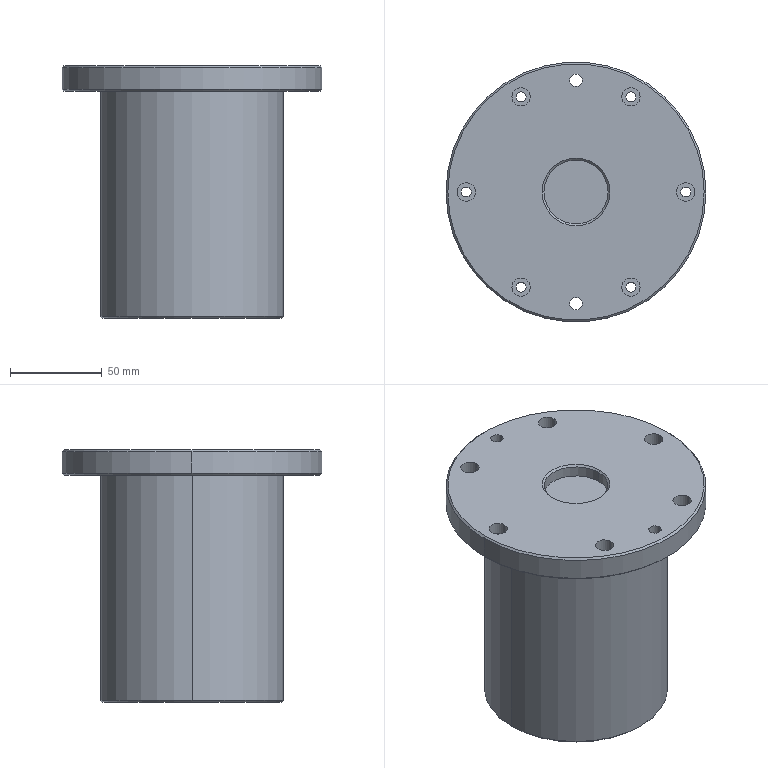Part | SolidWorks | features Chamfer 4, HoleWzd 2, ICE 2, CirPattern 1, Extrusion 1 | 1 solid | 52 faces | box 142 x 142 x 138 mm | volume 1182904 mm3 | cylinder 34 | plane 10 | cone 8 | commonest cylinder face diameters 5.5 x12 10 x12 6.8 x4 35 x2 100 x2 142 x2
STEP:
#1=CARTESIAN_POINT('',(-3.4,61.,124.));
#2=VERTEX_POINT('',#1);
#3=CARTESIAN_POINT('',(3.4,61.,124.));
#4=VERTEX_POINT('',#3);
#5=CARTESIAN_POINT('',(0.,61.,124.));
#6=DIRECTION('',(0.,0.,1.));
#7=DIRECTION('',(1.,0.,0.));
#8=AXIS2_PLACEMENT_3D('',#5,#6,#7);
#9=CIRCLE('',#8,3.4);
#10=EDGE_CURVE('',#2,#4,#9,.T.);
#11=ORIENTED_EDGE('',*,*,#10,.F.);
#12=CARTESIAN_POINT('',(-3.4,61.,138.));
#13=VERTEX_POINT('',#12);
#14=CARTESIAN_POINT('',(-3.4,61.,138.));
#15=DIRECTION('',(0.,0.,1.));
#16=VECTOR('',#15,1000.);
#17=LINE('',#14,#16);
#18=EDGE_CURVE('',#2,#13,#17,.T.);
#19=ORIENTED_EDGE('',*,*,#18,.T.);
#20=CARTESIAN_POINT('',(3.4,61.,138.));
#21=VERTEX_POINT('',#20);
#22=CARTESIAN_POINT('',(0.,61.,138.));
#23=DIRECTION('',(0.,0.,1.));
#24=DIRECTION('',(1.,0.,0.));
#25=AXIS2_PLACEMENT_3D('',#22,#23,#24);
#26=CIRCLE('',#25,3.4);
#27=EDGE_CURVE('',#13,#21,#26,.T.);
#28=ORIENTED_EDGE('',*,*,#27,.T.);
#29=CARTESIAN_POINT('',(3.4,61.,138.));
#30=DIRECTION('',(0.,0.,1.));
#31=VECTOR('',#30,1000.);
#32=LINE('',#29,#31);
#33=EDGE_CURVE('',#4,#21,#32,.T.);
#34=ORIENTED_EDGE('',*,*,#33,.F.);
#35=EDGE_LOOP('',(#11,#19,#28,#34));
#36=FACE_OUTER_BOUND('',#35,.T.);
#37=CARTESIAN_POINT('',(0.,61.,138.));
#38=DIRECTION('',(0.,0.,1.));
#39=DIRECTION('',(1.,0.,0.));
#40=AXIS2_PLACEMENT_3D('',#37,#38,#39);
#41=CYLINDRICAL_SURFACE('',#40,3.4);
#42=ADVANCED_FACE('',(#36),#41,.F.);
#43=CARTESIAN_POINT('',(-3.4,-61.,124.));
#44=VERTEX_POINT('',#43);
#45=CARTESIAN_POINT('',(3.4,-61.,124.));
#46=VERTEX_POINT('',#45);
#47=CARTESIAN_POINT('',(0.,-61.,124.));
#48=DIRECTION('',(0.,0.,1.));
#49=DIRECTION('',(1.,0.,0.));
#50=AXIS2_PLACEMENT_3D('',#47,#48,#49);
#51=CIRCLE('',#50,3.4);
#52=EDGE_CURVE('',#44,#46,#51,.T.);
#53=ORIENTED_EDGE('',*,*,#52,.F.);
#54=CARTESIAN_POINT('',(-3.4,-61.,138.));
#55=VERTEX_POINT('',#54);
#56=CARTESIAN_POINT('',(-3.4,-61.,138.));
#57=DIRECTION('',(0.,0.,1.));
#58=VECTOR('',#57,1000.);
#59=LINE('',#56,#58);
#60=EDGE_CURVE('',#44,#55,#59,.T.);
#61=ORIENTED_EDGE('',*,*,#60,.T.);
#62=CARTESIAN_POINT('',(3.4,-61.,138.));
#63=VERTEX_POINT('',#62);
#64=CARTESIAN_POINT('',(0.,-61.,138.));
#65=DIRECTION('',(0.,0.,1.));
#66=DIRECTION('',(1.,0.,0.));
#67=AXIS2_PLACEMENT_3D('',#64,#65,#66);
#68=CIRCLE('',#67,3.4);
#69=EDGE_CURVE('',#55,#63,#68,.T.);
#70=ORIENTED_EDGE('',*,*,#69,.T.);
#71=CARTESIAN_POINT('',(3.4,-61.,138.));
#72=DIRECTION('',(0.,0.,1.));
#73=VECTOR('',#72,1000.);
#74=LINE('',#71,#73);
#75=EDGE_CURVE('',#46,#63,#74,.T.);
#76=ORIENTED_EDGE('',*,*,#75,.F.);
#77=EDGE_LOOP('',(#53,#61,#70,#76));
#78=FACE_OUTER_BOUND('',#77,.T.);
#79=CARTESIAN_POINT('',(0.,-61.,138.));
#80=DIRECTION('',(0.,0.,1.));
#81=DIRECTION('',(1.,0.,0.));
#82=AXIS2_PLACEMENT_3D('',#79,#80,#81);
#83=CYLINDRICAL_SURFACE('',#82,3.4);
#84=ADVANCED_FACE('',(#78),#83,.F.);
#85=CARTESIAN_POINT('',(25.,51.962,131.));
#86=VERTEX_POINT('',#85);
#87=CARTESIAN_POINT('',(35.,51.962,131.));
#88=VERTEX_POINT('',#87);
#89=CARTESIAN_POINT('',(30.,51.962,131.));
#90=DIRECTION('',(0.,0.,1.));
#91=DIRECTION('',(1.,0.,0.));
#92=AXIS2_PLACEMENT_3D('',#89,#90,#91);
#93=CIRCLE('',#92,5.);
#94=EDGE_CURVE('',#86,#88,#93,.T.);
#95=ORIENTED_EDGE('',*,*,#94,.F.);
#96=CARTESIAN_POINT('',(25.,51.962,138.));
#97=VERTEX_POINT('',#96);
#98=CARTESIAN_POINT('',(25.,51.962,138.));
#99=DIRECTION('',(0.,0.,1.));
#100=VECTOR('',#99,1000.);
#101=LINE('',#98,#100);
#102=EDGE_CURVE('',#86,#97,#101,.T.);
#103=ORIENTED_EDGE('',*,*,#102,.T.);
#104=CARTESIAN_POINT('',(35.,51.962,138.));
#105=VERTEX_POINT('',#104);
#106=CARTESIAN_POINT('',(30.,51.962,138.));
#107=DIRECTION('',(0.,0.,1.));
#108=DIRECTION('',(1.,0.,0.));
#109=AXIS2_PLACEMENT_3D('',#106,#107,#108);
#110=CIRCLE('',#109,5.);
#111=EDGE_CURVE('',#97,#105,#110,.T.);
#112=ORIENTED_EDGE('',*,*,#111,.T.);
#113=CARTESIAN_POINT('',(35.,51.962,138.));
#114=DIRECTION('',(0.,0.,1.));
#115=VECTOR('',#114,1000.);
#116=LINE('',#113,#115);
#117=EDGE_CURVE('',#88,#105,#116,.T.);
#118=ORIENTED_EDGE('',*,*,#117,.F.);
#119=EDGE_LOOP('',(#95,#103,#112,#118));
#120=FACE_OUTER_BOUND('',#119,.T.);
#121=CARTESIAN_POINT('',(30.,51.962,138.));
#122=DIRECTION('',(0.,0.,1.));
#123=DIRECTION('',(1.,0.,0.));
#124=AXIS2_PLACEMENT_3D('',#121,#122,#123);
#125=CYLINDRICAL_SURFACE('',#124,5.);
#126=ADVANCED_FACE('',(#120),#125,.F.);
#127=CARTESIAN_POINT('',(27.25,51.962,124.));
#128=VERTEX_POINT('',#127);
#129=CARTESIAN_POINT('',(32.75,51.962,124.));
#130=VERTEX_POINT('',#129);
#131=CARTESIAN_POINT('',(30.,51.962,124.));
#132=DIRECTION('',(0.,0.,1.));
#133=DIRECTION('',(1.,0.,0.));
#134=AXIS2_PLACEMENT_3D('',#131,#132,#133);
#135=CIRCLE('',#134,2.75);
#136=EDGE_CURVE('',#128,#130,#135,.T.);
#137=ORIENTED_EDGE('',*,*,#136,.F.);
#138=CARTESIAN_POINT('',(27.25,51.962,131.));
#139=VERTEX_POINT('',#138);
#140=CARTESIAN_POINT('',(27.25,51.962,138.));
#141=DIRECTION('',(0.,0.,1.));
#142=VECTOR('',#141,1000.);
#143=LINE('',#140,#142);
#144=EDGE_CURVE('',#128,#139,#143,.T.);
#145=ORIENTED_EDGE('',*,*,#144,.T.);
#146=CARTESIAN_POINT('',(32.75,51.962,131.));
#147=VERTEX_POINT('',#146);
#148=CARTESIAN_POINT('',(30.,51.962,131.));
#149=DIRECTION('',(0.,0.,1.));
#150=DIRECTION('',(1.,0.,0.));
#151=AXIS2_PLACEMENT_3D('',#148,#149,#150);
#152=CIRCLE('',#151,2.75);
#153=EDGE_CURVE('',#139,#147,#152,.T.);
#154=ORIENTED_EDGE('',*,*,#153,.T.);
#155=CARTESIAN_POINT('',(32.75,51.962,138.));
#156=DIRECTION('',(0.,0.,1.));
#157=VECTOR('',#156,1000.);
#158=LINE('',#155,#157);
#159=EDGE_CURVE('',#130,#147,#158,.T.);
#160=ORIENTED_EDGE('',*,*,#159,.F.);
#161=EDGE_LOOP('',(#137,#145,#154,#160));
#162=FACE_OUTER_BOUND('',#161,.T.);
#163=CARTESIAN_POINT('',(30.,51.962,138.));
#164=DIRECTION('',(0.,0.,1.));
#165=DIRECTION('',(1.,0.,0.));
#166=AXIS2_PLACEMENT_3D('',#163,#164,#165);
#167=CYLINDRICAL_SURFACE('',#166,2.75);
#168=ADVANCED_FACE('',(#162),#167,.F.);
#169=CARTESIAN_POINT('',(-35.,51.962,131.));
#170=VERTEX_POINT('',#169);
#171=CARTESIAN_POINT('',(-25.,51.962,131.));
#172=VERTEX_POINT('',#171);
#173=CARTESIAN_POINT('',(-30.,51.962,131.));
#174=DIRECTION('',(0.,0.,1.));
#175=DIRECTION('',(1.,0.,0.));
#176=AXIS2_PLACEMENT_3D('',#173,#174,#175);
#177=CIRCLE('',#176,5.);
#178=EDGE_CURVE('',#170,#172,#177,.T.);
#179=ORIENTED_EDGE('',*,*,#178,.F.);
#180=CARTESIAN_POINT('',(-35.,51.962,138.));
#181=VERTEX_POINT('',#180);
#182=CARTESIAN_POINT('',(-35.,51.962,138.));
#183=DIRECTION('',(0.,0.,1.));
#184=VECTOR('',#183,1000.);
#185=LINE('',#182,#184);
#186=EDGE_CURVE('',#170,#181,#185,.T.);
#187=ORIENTED_EDGE('',*,*,#186,.T.);
#188=CARTESIAN_POINT('',(-25.,51.962,138.));
#189=VERTEX_POINT('',#188);
#190=CARTESIAN_POINT('',(-30.,51.962,138.));
#191=DIRECTION('',(0.,0.,1.));
#192=DIRECTION('',(1.,0.,0.));
#193=AXIS2_PLACEMENT_3D('',#190,#191,#192);
#194=CIRCLE('',#193,5.);
#195=EDGE_CURVE('',#181,#189,#194,.T.);
#196=ORIENTED_EDGE('',*,*,#195,.T.);
#197=CARTESIAN_POINT('',(-25.,51.962,138.));
#198=DIRECTION('',(0.,0.,1.));
#199=VECTOR('',#198,1000.);
#200=LINE('',#197,#199);
#201=EDGE_CURVE('',#172,#189,#200,.T.);
#202=ORIENTED_EDGE('',*,*,#201,.F.);
#203=EDGE_LOOP('',(#179,#187,#196,#202));
#204=FACE_OUTER_BOUND('',#203,.T.);
#205=CARTESIAN_POINT('',(-30.,51.962,138.));
#206=DIRECTION('',(0.,0.,1.));
#207=DIRECTION('',(1.,0.,0.));
#208=AXIS2_PLACEMENT_3D('',#205,#206,#207);
#209=CYLINDRICAL_SURFACE('',#208,5.);
#210=ADVANCED_FACE('',(#204),#209,.F.);
#211=CARTESIAN_POINT('',(-32.75,51.962,124.));
#212=VERTEX_POINT('',#211);
#213=CARTESIAN_POINT('',(-27.25,51.962,124.));
#214=VERTEX_POINT('',#213);
#215=CARTESIAN_POINT('',(-30.,51.962,124.));
#216=DIRECTION('',(0.,0.,1.));
#217=DIRECTION('',(1.,0.,0.));
#218=AXIS2_PLACEMENT_3D('',#215,#216,#217);
#219=CIRCLE('',#218,2.75);
#220=EDGE_CURVE('',#212,#214,#219,.T.);
#221=ORIENTED_EDGE('',*,*,#220,.F.);
#222=CARTESIAN_POINT('',(-32.75,51.962,131.));
#223=VERTEX_POINT('',#222);
#224=CARTESIAN_POINT('',(-32.75,51.962,138.));
#225=DIRECTION('',(0.,0.,1.));
#226=VECTOR('',#225,1000.);
#227=LINE('',#224,#226);
#228=EDGE_CURVE('',#212,#223,#227,.T.);
#229=ORIENTED_EDGE('',*,*,#228,.T.);
#230=CARTESIAN_POINT('',(-27.25,51.962,131.));
#231=VERTEX_POINT('',#230);
#232=CARTESIAN_POINT('',(-30.,51.962,131.));
#233=DIRECTION('',(0.,0.,1.));
#234=DIRECTION('',(1.,0.,0.));
#235=AXIS2_PLACEMENT_3D('',#232,#233,#234);
#236=CIRCLE('',#235,2.75);
#237=EDGE_CURVE('',#223,#231,#236,.T.);
#238=ORIENTED_EDGE('',*,*,#237,.T.);
#239=CARTESIAN_POINT('',(-27.25,51.962,138.));
#240=DIRECTION('',(0.,0.,1.));
#241=VECTOR('',#240,1000.);
#242=LINE('',#239,#241);
#243=EDGE_CURVE('',#214,#231,#242,.T.);
#244=ORIENTED_EDGE('',*,*,#243,.F.);
#245=EDGE_LOOP('',(#221,#229,#238,#244));
#246=FACE_OUTER_BOUND('',#245,.T.);
#247=CARTESIAN_POINT('',(-30.,51.962,138.));
#248=DIRECTION('',(0.,0.,1.));
#249=DIRECTION('',(1.,0.,0.));
#250=AXIS2_PLACEMENT_3D('',#247,#248,#249);
#251=CYLINDRICAL_SURFACE('',#250,2.75);
#252=ADVANCED_FACE('',(#246),#251,.F.);
#253=CARTESIAN_POINT('',(-65.,0.,131.));
#254=VERTEX_POINT('',#253);
#255=CARTESIAN_POINT('',(-55.,0.,131.));
#256=VERTEX_POINT('',#255);
#257=CARTESIAN_POINT('',(-60.,0.,131.));
#258=DIRECTION('',(0.,0.,1.));
#259=DIRECTION('',(1.,0.,0.));
#260=AXIS2_PLACEMENT_3D('',#257,#258,#259);
#261=CIRCLE('',#260,5.);
#262=EDGE_CURVE('',#254,#256,#261,.T.);
#263=ORIENTED_EDGE('',*,*,#262,.F.);
#264=CARTESIAN_POINT('',(-65.,0.,138.));
#265=VERTEX_POINT('',#264);
#266=CARTESIAN_POINT('',(-65.,0.,138.));
#267=DIRECTION('',(0.,0.,1.));
#268=VECTOR('',#267,1000.);
#269=LINE('',#266,#268);
#270=EDGE_CURVE('',#254,#265,#269,.T.);
#271=ORIENTED_EDGE('',*,*,#270,.T.);
#272=CARTESIAN_POINT('',(-55.,0.,138.));
#273=VERTEX_POINT('',#272);
#274=CARTESIAN_POINT('',(-60.,0.,138.));
#275=DIRECTION('',(0.,0.,1.));
#276=DIRECTION('',(1.,0.,0.));
#277=AXIS2_PLACEMENT_3D('',#274,#275,#276);
#278=CIRCLE('',#277,5.);
#279=EDGE_CURVE('',#265,#273,#278,.T.);
#280=ORIENTED_EDGE('',*,*,#279,.T.);
#281=CARTESIAN_POINT('',(-55.,0.,138.));
#282=DIRECTION('',(0.,0.,1.));
#283=VECTOR('',#282,1000.);
#284=LINE('',#281,#283);
#285=EDGE_CURVE('',#256,#273,#284,.T.);
#286=ORIENTED_EDGE('',*,*,#285,.F.);
#287=EDGE_LOOP('',(#263,#271,#280,#286));
#288=FACE_OUTER_BOUND('',#287,.T.);
#289=CARTESIAN_POINT('',(-60.,0.,138.));
#290=DIRECTION('',(0.,0.,1.));
#291=DIRECTION('',(1.,0.,0.));
#292=AXIS2_PLACEMENT_3D('',#289,#290,#291);
#293=CYLINDRICAL_SURFACE('',#292,5.);
#294=ADVANCED_FACE('',(#288),#293,.F.);
#295=CARTESIAN_POINT('',(-62.75,0.,124.));
#296=VERTEX_POINT('',#295);
#297=CARTESIAN_POINT('',(-57.25,0.,124.));
#298=VERTEX_POINT('',#297);
#299=CARTESIAN_POINT('',(-60.,0.,124.));
#300=DIRECTION('',(0.,0.,1.));
#301=DIRECTION('',(1.,0.,0.));
#302=AXIS2_PLACEMENT_3D('',#299,#300,#301);
#303=CIRCLE('',#302,2.75);
#304=EDGE_CURVE('',#296,#298,#303,.T.);
#305=ORIENTED_EDGE('',*,*,#304,.F.);
#306=CARTESIAN_POINT('',(-62.75,0.,131.));
#307=VERTEX_POINT('',#306);
#308=CARTESIAN_POINT('',(-62.75,0.,138.));
#309=DIRECTION('',(0.,0.,1.));
#310=VECTOR('',#309,1000.);
#311=LINE('',#308,#310);
#312=EDGE_CURVE('',#296,#307,#311,.T.);
#313=ORIENTED_EDGE('',*,*,#312,.T.);
#314=CARTESIAN_POINT('',(-57.25,0.,131.));
#315=VERTEX_POINT('',#314);
#316=CARTESIAN_POINT('',(-60.,0.,131.));
#317=DIRECTION('',(0.,0.,1.));
#318=DIRECTION('',(1.,0.,0.));
#319=AXIS2_PLACEMENT_3D('',#316,#317,#318);
#320=CIRCLE('',#319,2.75);
#321=EDGE_CURVE('',#307,#315,#320,.T.);
#322=ORIENTED_EDGE('',*,*,#321,.T.);
#323=CARTESIAN_POINT('',(-57.25,0.,138.));
#324=DIRECTION('',(0.,0.,1.));
#325=VECTOR('',#324,1000.);
#326=LINE('',#323,#325);
#327=EDGE_CURVE('',#298,#315,#326,.T.);
#328=ORIENTED_EDGE('',*,*,#327,.F.);
#329=EDGE_LOOP('',(#305,#313,#322,#328));
#330=FACE_OUTER_BOUND('',#329,.T.);
#331=CARTESIAN_POINT('',(-60.,0.,138.));
#332=DIRECTION('',(0.,0.,1.));
#333=DIRECTION('',(1.,0.,0.));
#334=AXIS2_PLACEMENT_3D('',#331,#332,#333);
#335=CYLINDRICAL_SURFACE('',#334,2.75);
#336=ADVANCED_FACE('',(#330),#335,.F.);
#337=CARTESIAN_POINT('',(-35.,-51.962,131.));
#338=VERTEX_POINT('',#337);
#339=CARTESIAN_POINT('',(-25.,-51.962,131.));
#340=VERTEX_POINT('',#339);
#341=CARTESIAN_POINT('',(-30.,-51.962,131.));
#342=DIRECTION('',(0.,0.,1.));
#343=DIRECTION('',(1.,0.,0.));
#344=AXIS2_PLACEMENT_3D('',#341,#342,#343);
#345=CIRCLE('',#344,5.);
#346=EDGE_CURVE('',#338,#340,#345,.T.);
#347=ORIENTED_EDGE('',*,*,#346,.F.);
#348=CARTESIAN_POINT('',(-35.,-51.962,138.));
#349=VERTEX_POINT('',#348);
#350=CARTESIAN_POINT('',(-35.,-51.962,138.));
#351=DIRECTION('',(0.,0.,1.));
#352=VECTOR('',#351,1000.);
#353=LINE('',#350,#352);
#354=EDGE_CURVE('',#338,#349,#353,.T.);
#355=ORIENTED_EDGE('',*,*,#354,.T.);
#356=CARTESIAN_POINT('',(-25.,-51.962,138.));
#357=VERTEX_POINT('',#356);
#358=CARTESIAN_POINT('',(-30.,-51.962,138.));
#359=DIRECTION('',(0.,0.,1.));
#360=DIRECTION('',(1.,0.,0.));
#361=AXIS2_PLACEMENT_3D('',#358,#359,#360);
#362=CIRCLE('',#361,5.);
#363=EDGE_CURVE('',#349,#357,#362,.T.);
#364=ORIENTED_EDGE('',*,*,#363,.T.);
#365=CARTESIAN_POINT('',(-25.,-51.962,138.));
#366=DIRECTION('',(0.,0.,1.));
#367=VECTOR('',#366,1000.);
#368=LINE('',#365,#367);
#369=EDGE_CURVE('',#340,#357,#368,.T.);
#370=ORIENTED_EDGE('',*,*,#369,.F.);
#371=EDGE_LOOP('',(#347,#355,#364,#370));
#372=FACE_OUTER_BOUND('',#371,.T.);
#373=CARTESIAN_POINT('',(-30.,-51.962,138.));
#374=DIRECTION('',(0.,0.,1.));
#375=DIRECTION('',(1.,0.,0.));
#376=AXIS2_PLACEMENT_3D('',#373,#374,#375);
#377=CYLINDRICAL_SURFACE('',#376,5.);
#378=ADVANCED_FACE('',(#372),#377,.F.);
#379=CARTESIAN_POINT('',(-32.75,-51.962,124.));
#380=VERTEX_POINT('',#379);
#381=CARTESIAN_POINT('',(-27.25,-51.962,124.));
#382=VERTEX_POINT('',#381);
#383=CARTESIAN_POINT('',(-30.,-51.962,124.));
#384=DIRECTION('',(0.,0.,1.));
#385=DIRECTION('',(1.,0.,0.));
#386=AXIS2_PLACEMENT_3D('',#383,#384,#385);
#387=CIRCLE('',#386,2.75);
#388=EDGE_CURVE('',#380,#382,#387,.T.);
#389=ORIENTED_EDGE('',*,*,#388,.F.);
#390=CARTESIAN_POINT('',(-32.75,-51.962,131.));
#391=VERTEX_POINT('',#390);
#392=CARTESIAN_POINT('',(-32.75,-51.962,138.));
#393=DIRECTION('',(0.,0.,1.));
#394=VECTOR('',#393,1000.);
#395=LINE('',#392,#394);
#396=EDGE_CURVE('',#380,#391,#395,.T.);
#397=ORIENTED_EDGE('',*,*,#396,.T.);
#398=CARTESIAN_POINT('',(-27.25,-51.962,131.));
#399=VERTEX_POINT('',#398);
#400=CARTESIAN_POINT('',(-30.,-51.962,131.));
#401=DIRECTION('',(0.,0.,1.));
#402=DIRECTION('',(1.,0.,0.));
#403=AXIS2_PLACEMENT_3D('',#400,#401,#402);
#404=CIRCLE('',#403,2.75);
#405=EDGE_CURVE('',#391,#399,#404,.T.);
#406=ORIENTED_EDGE('',*,*,#405,.T.);
#407=CARTESIAN_POINT('',(-27.25,-51.962,138.));
#408=DIRECTION('',(0.,0.,1.));
#409=VECTOR('',#408,1000.);
#410=LINE('',#407,#409);
#411=EDGE_CURVE('',#382,#399,#410,.T.);
#412=ORIENTED_EDGE('',*,*,#411,.F.);
#413=EDGE_LOOP('',(#389,#397,#406,#412));
#414=FACE_OUTER_BOUND('',#413,.T.);
#415=CARTESIAN_POINT('',(-30.,-51.962,138.));
#416=DIRECTION('',(0.,0.,1.));
#417=DIRECTION('',(1.,0.,0.));
#418=AXIS2_PLACEMENT_3D('',#415,#416,#417);
#419=CYLINDRICAL_SURFACE('',#418,2.75);
#420=ADVANCED_FACE('',(#414),#419,.F.);
#421=CARTESIAN_POINT('',(25.,-51.962,131.));
#422=VERTEX_POINT('',#421);
#423=CARTESIAN_POINT('',(35.,-51.962,131.));
#424=VERTEX_POINT('',#423);
#425=CARTESIAN_POINT('',(30.,-51.962,131.));
#426=DIRECTION('',(0.,0.,1.));
#427=DIRECTION('',(1.,0.,0.));
#428=AXIS2_PLACEMENT_3D('',#425,#426,#427);
#429=CIRCLE('',#428,5.);
#430=EDGE_CURVE('',#422,#424,#429,.T.);
#431=ORIENTED_EDGE('',*,*,#430,.F.);
#432=CARTESIAN_POINT('',(25.,-51.962,138.));
#433=VERTEX_POINT('',#432);
#434=CARTESIAN_POINT('',(25.,-51.962,138.));
#435=DIRECTION('',(0.,0.,1.));
#436=VECTOR('',#435,1000.);
#437=LINE('',#434,#436);
#438=EDGE_CURVE('',#422,#433,#437,.T.);
#439=ORIENTED_EDGE('',*,*,#438,.T.);
#440=CARTESIAN_POINT('',(35.,-51.962,138.));
#441=VERTEX_POINT('',#440);
#442=CARTESIAN_POINT('',(30.,-51.962,138.));
#443=DIRECTION('',(0.,0.,1.));
#444=DIRECTION('',(1.,0.,0.));
#445=AXIS2_PLACEMENT_3D('',#442,#443,#444);
#446=CIRCLE('',#445,5.);
#447=EDGE_CURVE('',#433,#441,#446,.T.);
#448=ORIENTED_EDGE('',*,*,#447,.T.);
#449=CARTESIAN_POINT('',(35.,-51.962,138.));
#450=DIRECTION('',(0.,0.,1.));
#451=VECTOR('',#450,1000.);
#452=LINE('',#449,#451);
#453=EDGE_CURVE('',#424,#441,#452,.T.);
#454=ORIENTED_EDGE('',*,*,#453,.F.);
#455=EDGE_LOOP('',(#431,#439,#448,#454));
#456=FACE_OUTER_BOUND('',#455,.T.);
#457=CARTESIAN_POINT('',(30.,-51.962,138.));
#458=DIRECTION('',(0.,0.,1.));
#459=DIRECTION('',(1.,0.,0.));
#460=AXIS2_PLACEMENT_3D('',#457,#458,#459);
#461=CYLINDRICAL_SURFACE('',#460,5.);
#462=ADVANCED_FACE('',(#456),#461,.F.);
#463=CARTESIAN_POINT('',(27.25,-51.962,124.));
#464=VERTEX_POINT('',#463);
#465=CARTESIAN_POINT('',(32.75,-51.962,124.));
#466=VERTEX_POINT('',#465);
#467=CARTESIAN_POINT('',(30.,-51.962,124.));
#468=DIRECTION('',(0.,0.,1.));
#469=DIRECTION('',(1.,0.,0.));
#470=AXIS2_PLACEMENT_3D('',#467,#468,#469);
#471=CIRCLE('',#470,2.75);
#472=EDGE_CURVE('',#464,#466,#471,.T.);
#473=ORIENTED_EDGE('',*,*,#472,.F.);
#474=CARTESIAN_POINT('',(27.25,-51.962,131.));
#475=VERTEX_POINT('',#474);
#476=CARTESIAN_POINT('',(27.25,-51.962,138.));
#477=DIRECTION('',(0.,0.,1.));
#478=VECTOR('',#477,1000.);
#479=LINE('',#476,#478);
#480=EDGE_CURVE('',#464,#475,#479,.T.);
#481=ORIENTED_EDGE('',*,*,#480,.T.);
#482=CARTESIAN_POINT('',(32.75,-51.962,131.));
#483=VERTEX_POINT('',#482);
#484=CARTESIAN_POINT('',(30.,-51.962,131.));
#485=DIRECTION('',(0.,0.,1.));
#486=DIRECTION('',(1.,0.,0.));
#487=AXIS2_PLACEMENT_3D('',#484,#485,#486);
#488=CIRCLE('',#487,2.75);
#489=EDGE_CURVE('',#475,#483,#488,.T.);
#490=ORIENTED_EDGE('',*,*,#489,.T.);
#491=CARTESIAN_POINT('',(32.75,-51.962,138.));
#492=DIRECTION('',(0.,0.,1.));
#493=VECTOR('',#492,1000.);
#494=LINE('',#491,#493);
#495=EDGE_CURVE('',#466,#483,#494,.T.);
#496=ORIENTED_EDGE('',*,*,#495,.F.);
#497=EDGE_LOOP('',(#473,#481,#490,#496));
#498=FACE_OUTER_BOUND('',#497,.T.);
#499=CARTESIAN_POINT('',(30.,-51.962,138.));
#500=DIRECTION('',(0.,0.,1.));
#501=DIRECTION('',(1.,0.,0.));
#502=AXIS2_PLACEMENT_3D('',#499,#500,#501);
#503=CYLINDRICAL_SURFACE('',#502,2.75);
#504=ADVANCED_FACE('',(#498),#503,.F.);
#505=CARTESIAN_POINT('',(55.,0.,131.));
#506=VERTEX_POINT('',#505);
#507=CARTESIAN_POINT('',(65.,0.,131.));
#508=VERTEX_POINT('',#507);
#509=CARTESIAN_POINT('',(60.,0.,131.));
#510=DIRECTION('',(0.,0.,1.));
#511=DIRECTION('',(1.,0.,0.));
#512=AXIS2_PLACEMENT_3D('',#509,#510,#511);
#513=CIRCLE('',#512,5.);
#514=EDGE_CURVE('',#506,#508,#513,.T.);
#515=ORIENTED_EDGE('',*,*,#514,.F.);
#516=CARTESIAN_POINT('',(55.,0.,138.));
#517=VERTEX_POINT('',#516);
#518=CARTESIAN_POINT('',(55.,0.,138.));
#519=DIRECTION('',(0.,0.,1.));
#520=VECTOR('',#519,1000.);
#521=LINE('',#518,#520);
#522=EDGE_CURVE('',#506,#517,#521,.T.);
#523=ORIENTED_EDGE('',*,*,#522,.T.);
#524=CARTESIAN_POINT('',(65.,0.,138.));
#525=VERTEX_POINT('',#524);
#526=CARTESIAN_POINT('',(60.,0.,138.));
#527=DIRECTION('',(0.,0.,1.));
#528=DIRECTION('',(1.,0.,0.));
#529=AXIS2_PLACEMENT_3D('',#526,#527,#528);
#530=CIRCLE('',#529,5.);
#531=EDGE_CURVE('',#517,#525,#530,.T.);
#532=ORIENTED_EDGE('',*,*,#531,.T.);
#533=CARTESIAN_POINT('',(65.,0.,138.));
#534=DIRECTION('',(0.,0.,1.));
#535=VECTOR('',#534,1000.);
#536=LINE('',#533,#535);
#537=EDGE_CURVE('',#508,#525,#536,.T.);
#538=ORIENTED_EDGE('',*,*,#537,.F.);
#539=EDGE_LOOP('',(#515,#523,#532,#538));
#540=FACE_OUTER_BOUND('',#539,.T.);
#541=CARTESIAN_POINT('',(60.,0.,138.));
#542=DIRECTION('',(0.,0.,1.));
#543=DIRECTION('',(1.,0.,0.));
#544=AXIS2_PLACEMENT_3D('',#541,#542,#543);
#545=CYLINDRICAL_SURFACE('',#544,5.);
#546=ADVANCED_FACE('',(#540),#545,.F.);
#547=CARTESIAN_POINT('',(57.25,0.,124.));
#548=VERTEX_POINT('',#547);
#549=CARTESIAN_POINT('',(62.75,0.,124.));
#550=VERTEX_POINT('',#549);
#551=CARTESIAN_POINT('',(60.,0.,124.));
#552=DIRECTION('',(0.,0.,1.));
#553=DIRECTION('',(1.,0.,0.));
#554=AXIS2_PLACEMENT_3D('',#551,#552,#553);
#555=CIRCLE('',#554,2.75);
#556=EDGE_CURVE('',#548,#550,#555,.T.);
#557=ORIENTED_EDGE('',*,*,#556,.F.);
#558=CARTESIAN_POINT('',(57.25,0.,131.));
#559=VERTEX_POINT('',#558);
#560=CARTESIAN_POINT('',(57.25,0.,138.));
#561=DIRECTION('',(0.,0.,1.));
#562=VECTOR('',#561,1000.);
#563=LINE('',#560,#562);
#564=EDGE_CURVE('',#548,#559,#563,.T.);
#565=ORIENTED_EDGE('',*,*,#564,.T.);
#566=CARTESIAN_POINT('',(62.75,0.,131.));
#567=VERTEX_POINT('',#566);
#568=CARTESIAN_POINT('',(60.,0.,131.));
#569=DIRECTION('',(0.,0.,1.));
#570=DIRECTION('',(1.,0.,0.));
#571=AXIS2_PLACEMENT_3D('',#568,#569,#570);
#572=CIRCLE('',#571,2.75);
#573=EDGE_CURVE('',#559,#567,#572,.T.);
#574=ORIENTED_EDGE('',*,*,#573,.T.);
#575=CARTESIAN_POINT('',(62.75,0.,138.));
#576=DIRECTION('',(0.,0.,1.));
#577=VECTOR('',#576,1000.);
#578=LINE('',#575,#577);
#579=EDGE_CURVE('',#550,#567,#578,.T.);
#580=ORIENTED_EDGE('',*,*,#579,.F.);
#581=EDGE_LOOP('',(#557,#565,#574,#580));
#582=FACE_OUTER_BOUND('',#581,.T.);
#583=CARTESIAN_POINT('',(60.,0.,138.));
#584=DIRECTION('',(0.,0.,1.));
#585=DIRECTION('',(1.,0.,0.));
#586=AXIS2_PLACEMENT_3D('',#583,#584,#585);
#587=CYLINDRICAL_SURFACE('',#586,2.75);
#588=ADVANCED_FACE('',(#582),#587,.F.);
#589=CARTESIAN_POINT('',(-17.5,0.,137.));
#590=VERTEX_POINT('',#589);
#591=CARTESIAN_POINT('',(17.5,0.,137.));
#592=VERTEX_POINT('',#591);
#593=CARTESIAN_POINT('',(0.,0.,137.));
#594=DIRECTION('',(0.,0.,1.));
#595=DIRECTION('',(1.,0.,0.));
#596=AXIS2_PLACEMENT_3D('',#593,#594,#595);
#597=CIRCLE('',#596,17.5);
#598=EDGE_CURVE('',#590,#592,#597,.T.);
#599=ORIENTED_EDGE('',*,*,#598,.F.);
#600=CARTESIAN_POINT('',(-18.5,0.,138.));
#601=VERTEX_POINT('',#600);
#602=CARTESIAN_POINT('',(-17.5,0.,137.));
#603=DIRECTION('',(-0.7071,0.,0.7071));
#604=VECTOR('',#603,1000.);
#605=LINE('',#602,#604);
#606=EDGE_CURVE('',#590,#601,#605,.T.);
#607=ORIENTED_EDGE('',*,*,#606,.T.);
#608=CARTESIAN_POINT('',(18.5,0.,138.));
#609=VERTEX_POINT('',#608);
#610=CARTESIAN_POINT('',(0.,0.,138.));
#611=DIRECTION('',(0.,0.,-1.));
#612=DIRECTION('',(1.,0.,0.));
#613=AXIS2_PLACEMENT_3D('',#610,#611,#612);
#614=CIRCLE('',#613,18.5);
#615=EDGE_CURVE('',#609,#601,#614,.T.);
#616=ORIENTED_EDGE('',*,*,#615,.F.);
#617=CARTESIAN_POINT('',(17.5,0.,137.));
#618=DIRECTION('',(0.7071,0.,0.7071));
#619=VECTOR('',#618,1000.);
#620=LINE('',#617,#619);
#621=EDGE_CURVE('',#592,#609,#620,.T.);
#622=ORIENTED_EDGE('',*,*,#621,.F.);
#623=EDGE_LOOP('',(#599,#607,#616,#622));
#624=FACE_OUTER_BOUND('',#623,.T.);
#625=CARTESIAN_POINT('',(0.,0.,137.));
#626=DIRECTION('',(0.,0.,1.));
#627=DIRECTION('',(1.,0.,0.));
#628=AXIS2_PLACEMENT_3D('',#625,#626,#627);
#629=CONICAL_SURFACE('',#628,17.5,0.7854);
#630=ADVANCED_FACE('',(#624),#629,.F.);
#631=CARTESIAN_POINT('',(-17.5,0.,131.));
#632=VERTEX_POINT('',#631);
#633=CARTESIAN_POINT('',(17.5,0.,131.));
#634=VERTEX_POINT('',#633);
#635=CARTESIAN_POINT('',(0.,0.,131.));
#636=DIRECTION('',(0.,0.,1.));
#637=DIRECTION('',(1.,0.,0.));
#638=AXIS2_PLACEMENT_3D('',#635,#636,#637);
#639=CIRCLE('',#638,17.5);
#640=EDGE_CURVE('',#632,#634,#639,.T.);
#641=ORIENTED_EDGE('',*,*,#640,.F.);
#642=CARTESIAN_POINT('',(-17.5,0.,131.));
#643=DIRECTION('',(0.,0.,1.));
#644=VECTOR('',#643,1000.);
#645=LINE('',#642,#644);
#646=EDGE_CURVE('',#632,#590,#645,.T.);
#647=ORIENTED_EDGE('',*,*,#646,.T.);
#648=ORIENTED_EDGE('',*,*,#598,.T.);
#649=CARTESIAN_POINT('',(17.5,0.,131.));
#650=DIRECTION('',(0.,0.,1.));
#651=VECTOR('',#650,1000.);
#652=LINE('',#649,#651);
#653=EDGE_CURVE('',#634,#592,#652,.T.);
#654=ORIENTED_EDGE('',*,*,#653,.F.);
#655=EDGE_LOOP('',(#641,#647,#648,#654));
#656=FACE_OUTER_BOUND('',#655,.T.);
#657=CARTESIAN_POINT('',(0.,0.,131.));
#658=DIRECTION('',(0.,0.,1.));
#659=DIRECTION('',(1.,0.,0.));
#660=AXIS2_PLACEMENT_3D('',#657,#658,#659);
#661=CYLINDRICAL_SURFACE('',#660,17.5);
#662=ADVANCED_FACE('',(#656),#661,.F.);
#663=CARTESIAN_POINT('',(-70.,0.,124.));
#664=VERTEX_POINT('',#663);
#665=CARTESIAN_POINT('',(70.,0.,124.));
#666=VERTEX_POINT('',#665);
#667=CARTESIAN_POINT('',(0.,0.,124.));
#668=DIRECTION('',(0.,0.,-1.));
#669=DIRECTION('',(1.,0.,0.));
#670=AXIS2_PLACEMENT_3D('',#667,#668,#669);
#671=CIRCLE('',#670,70.);
#672=EDGE_CURVE('',#664,#666,#671,.T.);
#673=ORIENTED_EDGE('',*,*,#672,.F.);
#674=CARTESIAN_POINT('',(-71.,0.,125.));
#675=VERTEX_POINT('',#674);
#676=CARTESIAN_POINT('',(-71.,0.,125.));
#677=DIRECTION('',(-0.7071,0.,0.7071));
#678=VECTOR('',#677,1000.);
#679=LINE('',#676,#678);
#680=EDGE_CURVE('',#664,#675,#679,.T.);
#681=ORIENTED_EDGE('',*,*,#680,.T.);
#682=CARTESIAN_POINT('',(71.,0.,125.));
#683=VERTEX_POINT('',#682);
#684=CARTESIAN_POINT('',(0.,0.,125.));
#685=DIRECTION('',(0.,0.,1.));
#686=DIRECTION('',(1.,0.,0.));
#687=AXIS2_PLACEMENT_3D('',#684,#685,#686);
#688=CIRCLE('',#687,71.);
#689=EDGE_CURVE('',#683,#675,#688,.T.);
#690=ORIENTED_EDGE('',*,*,#689,.F.);
#691=CARTESIAN_POINT('',(71.,0.,125.));
#692=DIRECTION('',(0.7071,0.,0.7071));
#693=VECTOR('',#692,1000.);
#694=LINE('',#691,#693);
#695=EDGE_CURVE('',#666,#683,#694,.T.);
#696=ORIENTED_EDGE('',*,*,#695,.F.);
#697=EDGE_LOOP('',(#673,#681,#690,#696));
#698=FACE_OUTER_BOUND('',#697,.T.);
#699=CARTESIAN_POINT('',(0.,0.,125.));
#700=DIRECTION('',(0.,0.,1.));
#701=DIRECTION('',(1.,0.,0.));
#702=AXIS2_PLACEMENT_3D('',#699,#700,#701);
#703=CONICAL_SURFACE('',#702,71.,0.7854);
#704=ADVANCED_FACE('',(#698),#703,.T.);
#705=CARTESIAN_POINT('',(70.,0.,138.));
#706=VERTEX_POINT('',#705);
#707=CARTESIAN_POINT('',(-70.,0.,138.));
#708=VERTEX_POINT('',#707);
#709=CARTESIAN_POINT('',(0.,0.,138.));
#710=DIRECTION('',(0.,0.,1.));
#711=DIRECTION('',(1.,0.,0.));
#712=AXIS2_PLACEMENT_3D('',#709,#710,#711);
#713=CIRCLE('',#712,70.);
#714=EDGE_CURVE('',#706,#708,#713,.T.);
#715=ORIENTED_EDGE('',*,*,#714,.F.);
#716=CARTESIAN_POINT('',(71.,0.,137.));
#717=VERTEX_POINT('',#716);
#718=CARTESIAN_POINT('',(70.,0.,138.));
#719=DIRECTION('',(0.7071,0.,-0.7071));
#720=VECTOR('',#719,1000.);
#721=LINE('',#718,#720);
#722=EDGE_CURVE('',#706,#717,#721,.T.);
#723=ORIENTED_EDGE('',*,*,#722,.T.);
#724=CARTESIAN_POINT('',(-71.,0.,137.));
#725=VERTEX_POINT('',#724);
#726=CARTESIAN_POINT('',(0.,0.,137.));
#727=DIRECTION('',(0.,0.,-1.));
#728=DIRECTION('',(1.,0.,0.));
#729=AXIS2_PLACEMENT_3D('',#726,#727,#728);
#730=CIRCLE('',#729,71.);
#731=EDGE_CURVE('',#725,#717,#730,.T.);
#732=ORIENTED_EDGE('',*,*,#731,.F.);
#733=CARTESIAN_POINT('',(-70.,0.,138.));
#734=DIRECTION('',(-0.7071,0.,-0.7071));
#735=VECTOR('',#734,1000.);
#736=LINE('',#733,#735);
#737=EDGE_CURVE('',#708,#725,#736,.T.);
#738=ORIENTED_EDGE('',*,*,#737,.F.);
#739=EDGE_LOOP('',(#715,#723,#732,#738));
#740=FACE_OUTER_BOUND('',#739,.T.);
#741=CARTESIAN_POINT('',(0.,0.,138.));
#742=DIRECTION('',(0.,0.,-1.));
#743=DIRECTION('',(-1.,0.,0.));
#744=AXIS2_PLACEMENT_3D('',#741,#742,#743);
#745=CONICAL_SURFACE('',#744,70.,0.7854);
#746=ADVANCED_FACE('',(#740),#745,.T.);
#747=CARTESIAN_POINT('',(-49.,0.,0.));
#748=VERTEX_POINT('',#747);
#749=CARTESIAN_POINT('',(49.,0.,0.));
#750=VERTEX_POINT('',#749);
#751=CARTESIAN_POINT('',(0.,0.,0.));
#752=DIRECTION('',(0.,0.,-1.));
#753=DIRECTION('',(1.,0.,0.));
#754=AXIS2_PLACEMENT_3D('',#751,#752,#753);
#755=CIRCLE('',#754,49.);
#756=EDGE_CURVE('',#748,#750,#755,.T.);
#757=ORIENTED_EDGE('',*,*,#756,.F.);
#758=CARTESIAN_POINT('',(-50.,0.,1.));
#759=VERTEX_POINT('',#758);
#760=CARTESIAN_POINT('',(-50.,0.,1.));
#761=DIRECTION('',(-0.7071,0.,0.7071));
#762=VECTOR('',#761,1000.);
#763=LINE('',#760,#762);
#764=EDGE_CURVE('',#748,#759,#763,.T.);
#765=ORIENTED_EDGE('',*,*,#764,.T.);
#766=CARTESIAN_POINT('',(50.,0.,1.));
#767=VERTEX_POINT('',#766);
#768=CARTESIAN_POINT('',(0.,0.,1.));
#769=DIRECTION('',(0.,0.,1.));
#770=DIRECTION('',(1.,0.,0.));
#771=AXIS2_PLACEMENT_3D('',#768,#769,#770);
#772=CIRCLE('',#771,50.);
#773=EDGE_CURVE('',#767,#759,#772,.T.);
#774=ORIENTED_EDGE('',*,*,#773,.F.);
#775=CARTESIAN_POINT('',(50.,0.,1.));
#776=DIRECTION('',(0.7071,0.,0.7071));
#777=VECTOR('',#776,1000.);
#778=LINE('',#775,#777);
#779=EDGE_CURVE('',#750,#767,#778,.T.);
#780=ORIENTED_EDGE('',*,*,#779,.F.);
#781=EDGE_LOOP('',(#757,#765,#774,#780));
#782=FACE_OUTER_BOUND('',#781,.T.);
#783=CARTESIAN_POINT('',(0.,0.,1.));
#784=DIRECTION('',(0.,0.,1.));
#785=DIRECTION('',(1.,0.,0.));
#786=AXIS2_PLACEMENT_3D('',#783,#784,#785);
#787=CONICAL_SURFACE('',#786,50.,0.7854);
#788=ADVANCED_FACE('',(#782),#787,.T.);
#789=ORIENTED_EDGE('',*,*,#689,.T.);
#790=CARTESIAN_POINT('',(-71.,0.,124.));
#791=DIRECTION('',(0.,0.,1.));
#792=VECTOR('',#791,1000.);
#793=LINE('',#790,#792);
#794=EDGE_CURVE('',#675,#725,#793,.T.);
#795=ORIENTED_EDGE('',*,*,#794,.T.);
#796=ORIENTED_EDGE('',*,*,#731,.T.);
#797=CARTESIAN_POINT('',(71.,0.,124.));
#798=DIRECTION('',(0.,0.,1.));
#799=VECTOR('',#798,1000.);
#800=LINE('',#797,#799);
#801=EDGE_CURVE('',#683,#717,#800,.T.);
#802=ORIENTED_EDGE('',*,*,#801,.F.);
#803=EDGE_LOOP('',(#789,#795,#796,#802));
#804=FACE_OUTER_BOUND('',#803,.T.);
#805=CARTESIAN_POINT('',(0.,0.,124.));
#806=DIRECTION('',(0.,0.,1.));
#807=DIRECTION('',(1.,0.,0.));
#808=AXIS2_PLACEMENT_3D('',#805,#806,#807);
#809=CYLINDRICAL_SURFACE('',#808,71.);
#810=ADVANCED_FACE('',(#804),#809,.T.);
#811=CARTESIAN_POINT('',(50.,0.,124.));
#812=VERTEX_POINT('',#811);
#813=CARTESIAN_POINT('',(-50.,0.,124.));
#814=VERTEX_POINT('',#813);
#815=CARTESIAN_POINT('',(0.,0.,124.));
#816=DIRECTION('',(0.,0.,1.));
#817=DIRECTION('',(1.,0.,0.));
#818=AXIS2_PLACEMENT_3D('',#815,#816,#817);
#819=CIRCLE('',#818,50.);
#820=EDGE_CURVE('',#812,#814,#819,.T.);
#821=ORIENTED_EDGE('',*,*,#820,.F.);
#822=CARTESIAN_POINT('',(50.,0.,138.));
#823=DIRECTION('',(0.,0.,-1.));
#824=VECTOR('',#823,1000.);
#825=LINE('',#822,#824);
#826=EDGE_CURVE('',#812,#767,#825,.T.);
#827=ORIENTED_EDGE('',*,*,#826,.T.);
#828=ORIENTED_EDGE('',*,*,#773,.T.);
#829=CARTESIAN_POINT('',(-50.,0.,138.));
#830=DIRECTION('',(0.,0.,-1.));
#831=VECTOR('',#830,1000.);
#832=LINE('',#829,#831);
#833=EDGE_CURVE('',#814,#759,#832,.T.);
#834=ORIENTED_EDGE('',*,*,#833,.F.);
#835=EDGE_LOOP('',(#821,#827,#828,#834));
#836=FACE_OUTER_BOUND('',#835,.T.);
#837=CARTESIAN_POINT('',(0.,0.,138.));
#838=DIRECTION('',(0.,0.,-1.));
#839=DIRECTION('',(-1.,0.,0.));
#840=AXIS2_PLACEMENT_3D('',#837,#838,#839);
#841=CYLINDRICAL_SURFACE('',#840,50.);
#842=ADVANCED_FACE('',(#836),#841,.T.);
#843=ORIENTED_EDGE('',*,*,#826,.F.);
#844=CARTESIAN_POINT('',(0.,0.,124.));
#845=DIRECTION('',(0.,0.,1.));
#846=DIRECTION('',(1.,0.,0.));
#847=AXIS2_PLACEMENT_3D('',#844,#845,#846);
#848=CIRCLE('',#847,50.);
#849=EDGE_CURVE('',#814,#812,#848,.T.);
#850=ORIENTED_EDGE('',*,*,#849,.F.);
#851=ORIENTED_EDGE('',*,*,#833,.T.);
#852=CARTESIAN_POINT('',(0.,0.,1.));
#853=DIRECTION('',(0.,0.,1.));
#854=DIRECTION('',(1.,0.,0.));
#855=AXIS2_PLACEMENT_3D('',#852,#853,#854);
#856=CIRCLE('',#855,50.);
#857=EDGE_CURVE('',#759,#767,#856,.T.);
#858=ORIENTED_EDGE('',*,*,#857,.T.);
#859=EDGE_LOOP('',(#843,#850,#851,#858));
#860=FACE_OUTER_BOUND('',#859,.T.);
#861=CARTESIAN_POINT('',(0.,0.,138.));
#862=DIRECTION('',(0.,0.,-1.));
#863=DIRECTION('',(-1.,0.,0.));
#864=AXIS2_PLACEMENT_3D('',#861,#862,#863);
#865=CYLINDRICAL_SURFACE('',#864,50.);
#866=ADVANCED_FACE('',(#860),#865,.T.);
#867=CARTESIAN_POINT('',(0.,0.,0.));
#868=DIRECTION('',(0.,0.,-1.));
#869=DIRECTION('',(1.,0.,0.));
#870=AXIS2_PLACEMENT_3D('',#867,#868,#869);
#871=CIRCLE('',#870,49.);
#872=EDGE_CURVE('',#750,#748,#871,.T.);
#873=ORIENTED_EDGE('',*,*,#872,.T.);
#874=ORIENTED_EDGE('',*,*,#756,.T.);
#875=EDGE_LOOP('',(#873,#874));
#876=FACE_OUTER_BOUND('',#875,.T.);
#877=CARTESIAN_POINT('',(0.,0.,0.));
#878=DIRECTION('',(0.,0.,1.));
#879=DIRECTION('',(1.,0.,0.));
#880=AXIS2_PLACEMENT_3D('',#877,#878,#879);
#881=PLANE('',#880);
#882=ADVANCED_FACE('',(#876),#881,.F.);
#883=ORIENTED_EDGE('',*,*,#794,.F.);
#884=CARTESIAN_POINT('',(0.,0.,125.));
#885=DIRECTION('',(0.,0.,1.));
#886=DIRECTION('',(1.,0.,0.));
#887=AXIS2_PLACEMENT_3D('',#884,#885,#886);
#888=CIRCLE('',#887,71.);
#889=EDGE_CURVE('',#675,#683,#888,.T.);
#890=ORIENTED_EDGE('',*,*,#889,.T.);
#891=ORIENTED_EDGE('',*,*,#801,.T.);
#892=CARTESIAN_POINT('',(0.,0.,137.));
#893=DIRECTION('',(0.,0.,-1.));
#894=DIRECTION('',(1.,0.,0.));
#895=AXIS2_PLACEMENT_3D('',#892,#893,#894);
#896=CIRCLE('',#895,71.);
#897=EDGE_CURVE('',#717,#725,#896,.T.);
#898=ORIENTED_EDGE('',*,*,#897,.T.);
#899=EDGE_LOOP('',(#883,#890,#891,#898));
#900=FACE_OUTER_BOUND('',#899,.T.);
#901=CARTESIAN_POINT('',(0.,0.,124.));
#902=DIRECTION('',(0.,0.,1.));
#903=DIRECTION('',(1.,0.,0.));
#904=AXIS2_PLACEMENT_3D('',#901,#902,#903);
#905=CYLINDRICAL_SURFACE('',#904,71.);
#906=ADVANCED_FACE('',(#900),#905,.T.);
#907=CARTESIAN_POINT('',(0.,61.,124.));
#908=DIRECTION('',(0.,0.,1.));
#909=DIRECTION('',(1.,0.,0.));
#910=AXIS2_PLACEMENT_3D('',#907,#908,#909);
#911=CIRCLE('',#910,3.4);
#912=EDGE_CURVE('',#4,#2,#911,.T.);
#913=ORIENTED_EDGE('',*,*,#912,.T.);
#914=ORIENTED_EDGE('',*,*,#10,.T.);
#915=EDGE_LOOP('',(#913,#914));
#916=FACE_BOUND('',#915,.T.);
#917=CARTESIAN_POINT('',(0.,-61.,124.));
#918=DIRECTION('',(0.,0.,1.));
#919=DIRECTION('',(1.,0.,0.));
#920=AXIS2_PLACEMENT_3D('',#917,#918,#919);
#921=CIRCLE('',#920,3.4);
#922=EDGE_CURVE('',#46,#44,#921,.T.);
#923=ORIENTED_EDGE('',*,*,#922,.T.);
#924=ORIENTED_EDGE('',*,*,#52,.T.);
#925=EDGE_LOOP('',(#923,#924));
#926=FACE_BOUND('',#925,.T.);
#927=CARTESIAN_POINT('',(30.,51.962,124.));
#928=DIRECTION('',(0.,0.,1.));
#929=DIRECTION('',(1.,0.,0.));
#930=AXIS2_PLACEMENT_3D('',#927,#928,#929);
#931=CIRCLE('',#930,2.75);
#932=EDGE_CURVE('',#130,#128,#931,.T.);
#933=ORIENTED_EDGE('',*,*,#932,.T.);
#934=ORIENTED_EDGE('',*,*,#136,.T.);
#935=EDGE_LOOP('',(#933,#934));
#936=FACE_BOUND('',#935,.T.);
#937=CARTESIAN_POINT('',(-30.,51.962,124.));
#938=DIRECTION('',(0.,0.,1.));
#939=DIRECTION('',(1.,0.,0.));
#940=AXIS2_PLACEMENT_3D('',#937,#938,#939);
#941=CIRCLE('',#940,2.75);
#942=EDGE_CURVE('',#214,#212,#941,.T.);
#943=ORIENTED_EDGE('',*,*,#942,.T.);
#944=ORIENTED_EDGE('',*,*,#220,.T.);
#945=EDGE_LOOP('',(#943,#944));
#946=FACE_BOUND('',#945,.T.);
#947=CARTESIAN_POINT('',(-60.,0.,124.));
#948=DIRECTION('',(0.,0.,1.));
#949=DIRECTION('',(1.,0.,0.));
#950=AXIS2_PLACEMENT_3D('',#947,#948,#949);
#951=CIRCLE('',#950,2.75);
#952=EDGE_CURVE('',#298,#296,#951,.T.);
#953=ORIENTED_EDGE('',*,*,#952,.T.);
#954=ORIENTED_EDGE('',*,*,#304,.T.);
#955=EDGE_LOOP('',(#953,#954));
#956=FACE_BOUND('',#955,.T.);
#957=CARTESIAN_POINT('',(-30.,-51.962,124.));
#958=DIRECTION('',(0.,0.,1.));
#959=DIRECTION('',(1.,0.,0.));
#960=AXIS2_PLACEMENT_3D('',#957,#958,#959);
#961=CIRCLE('',#960,2.75);
#962=EDGE_CURVE('',#382,#380,#961,.T.);
#963=ORIENTED_EDGE('',*,*,#962,.T.);
#964=ORIENTED_EDGE('',*,*,#388,.T.);
#965=EDGE_LOOP('',(#963,#964));
#966=FACE_BOUND('',#965,.T.);
#967=CARTESIAN_POINT('',(30.,-51.962,124.));
#968=DIRECTION('',(0.,0.,1.));
#969=DIRECTION('',(1.,0.,0.));
#970=AXIS2_PLACEMENT_3D('',#967,#968,#969);
#971=CIRCLE('',#970,2.75);
#972=EDGE_CURVE('',#466,#464,#971,.T.);
#973=ORIENTED_EDGE('',*,*,#972,.T.);
#974=ORIENTED_EDGE('',*,*,#472,.T.);
#975=EDGE_LOOP('',(#973,#974));
#976=FACE_BOUND('',#975,.T.);
#977=CARTESIAN_POINT('',(60.,0.,124.));
#978=DIRECTION('',(0.,0.,1.));
#979=DIRECTION('',(1.,0.,0.));
#980=AXIS2_PLACEMENT_3D('',#977,#978,#979);
#981=CIRCLE('',#980,2.75);
#982=EDGE_CURVE('',#550,#548,#981,.T.);
#983=ORIENTED_EDGE('',*,*,#982,.T.);
#984=ORIENTED_EDGE('',*,*,#556,.T.);
#985=EDGE_LOOP('',(#983,#984));
#986=FACE_BOUND('',#985,.T.);
#987=CARTESIAN_POINT('',(0.,0.,124.));
#988=DIRECTION('',(0.,0.,-1.));
#989=DIRECTION('',(1.,0.,0.));
#990=AXIS2_PLACEMENT_3D('',#987,#988,#989);
#991=CIRCLE('',#990,70.);
#992=EDGE_CURVE('',#666,#664,#991,.T.);
#993=ORIENTED_EDGE('',*,*,#992,.T.);
#994=ORIENTED_EDGE('',*,*,#672,.T.);
#995=EDGE_LOOP('',(#993,#994));
#996=FACE_OUTER_BOUND('',#995,.T.);
#997=ORIENTED_EDGE('',*,*,#849,.T.);
#998=ORIENTED_EDGE('',*,*,#820,.T.);
#999=EDGE_LOOP('',(#997,#998));
#1000=FACE_BOUND('',#999,.T.);
#1001=CARTESIAN_POINT('',(0.,0.,124.));
#1002=DIRECTION('',(0.,0.,1.));
#1003=DIRECTION('',(1.,0.,0.));
#1004=AXIS2_PLACEMENT_3D('',#1001,#1002,#1003);
#1005=PLANE('',#1004);
#1006=ADVANCED_FACE('',(#916,#926,#936,#946,#956,#966,#976,#986,#996,#1000),#1005,.F.);
#1007=CARTESIAN_POINT('',(0.,61.,138.));
#1008=DIRECTION('',(0.,0.,1.));
#1009=DIRECTION('',(1.,0.,0.));
#1010=AXIS2_PLACEMENT_3D('',#1007,#1008,#1009);
#1011=CIRCLE('',#1010,3.4);
#1012=EDGE_CURVE('',#21,#13,#1011,.T.);
#1013=ORIENTED_EDGE('',*,*,#1012,.F.);
#1014=ORIENTED_EDGE('',*,*,#27,.F.);
#1015=EDGE_LOOP('',(#1013,#1014));
#1016=FACE_BOUND('',#1015,.T.);
#1017=CARTESIAN_POINT('',(0.,-61.,138.));
#1018=DIRECTION('',(0.,0.,1.));
#1019=DIRECTION('',(1.,0.,0.));
#1020=AXIS2_PLACEMENT_3D('',#1017,#1018,#1019);
#1021=CIRCLE('',#1020,3.4);
#1022=EDGE_CURVE('',#63,#55,#1021,.T.);
#1023=ORIENTED_EDGE('',*,*,#1022,.F.);
#1024=ORIENTED_EDGE('',*,*,#69,.F.);
#1025=EDGE_LOOP('',(#1023,#1024));
#1026=FACE_BOUND('',#1025,.T.);
#1027=CARTESIAN_POINT('',(30.,51.962,138.));
#1028=DIRECTION('',(0.,0.,1.));
#1029=DIRECTION('',(1.,0.,0.));
#1030=AXIS2_PLACEMENT_3D('',#1027,#1028,#1029);
#1031=CIRCLE('',#1030,5.);
#1032=EDGE_CURVE('',#105,#97,#1031,.T.);
#1033=ORIENTED_EDGE('',*,*,#1032,.F.);
#1034=ORIENTED_EDGE('',*,*,#111,.F.);
#1035=EDGE_LOOP('',(#1033,#1034));
#1036=FACE_BOUND('',#1035,.T.);
#1037=CARTESIAN_POINT('',(-30.,51.962,138.));
#1038=DIRECTION('',(0.,0.,1.));
#1039=DIRECTION('',(1.,0.,0.));
#1040=AXIS2_PLACEMENT_3D('',#1037,#1038,#1039);
#1041=CIRCLE('',#1040,5.);
#1042=EDGE_CURVE('',#189,#181,#1041,.T.);
#1043=ORIENTED_EDGE('',*,*,#1042,.F.);
#1044=ORIENTED_EDGE('',*,*,#195,.F.);
#1045=EDGE_LOOP('',(#1043,#1044));
#1046=FACE_BOUND('',#1045,.T.);
#1047=CARTESIAN_POINT('',(-60.,0.,138.));
#1048=DIRECTION('',(0.,0.,1.));
#1049=DIRECTION('',(1.,0.,0.));
#1050=AXIS2_PLACEMENT_3D('',#1047,#1048,#1049);
#1051=CIRCLE('',#1050,5.);
#1052=EDGE_CURVE('',#273,#265,#1051,.T.);
#1053=ORIENTED_EDGE('',*,*,#1052,.F.);
#1054=ORIENTED_EDGE('',*,*,#279,.F.);
#1055=EDGE_LOOP('',(#1053,#1054));
#1056=FACE_BOUND('',#1055,.T.);
#1057=CARTESIAN_POINT('',(-30.,-51.962,138.));
#1058=DIRECTION('',(0.,0.,1.));
#1059=DIRECTION('',(1.,0.,0.));
#1060=AXIS2_PLACEMENT_3D('',#1057,#1058,#1059);
#1061=CIRCLE('',#1060,5.);
#1062=EDGE_CURVE('',#357,#349,#1061,.T.);
#1063=ORIENTED_EDGE('',*,*,#1062,.F.);
#1064=ORIENTED_EDGE('',*,*,#363,.F.);
#1065=EDGE_LOOP('',(#1063,#1064));
#1066=FACE_BOUND('',#1065,.T.);
#1067=CARTESIAN_POINT('',(30.,-51.962,138.));
#1068=DIRECTION('',(0.,0.,1.));
#1069=DIRECTION('',(1.,0.,0.));
#1070=AXIS2_PLACEMENT_3D('',#1067,#1068,#1069);
#1071=CIRCLE('',#1070,5.);
#1072=EDGE_CURVE('',#441,#433,#1071,.T.);
#1073=ORIENTED_EDGE('',*,*,#1072,.F.);
#1074=ORIENTED_EDGE('',*,*,#447,.F.);
#1075=EDGE_LOOP('',(#1073,#1074));
#1076=FACE_BOUND('',#1075,.T.);
#1077=CARTESIAN_POINT('',(60.,0.,138.));
#1078=DIRECTION('',(0.,0.,1.));
#1079=DIRECTION('',(1.,0.,0.));
#1080=AXIS2_PLACEMENT_3D('',#1077,#1078,#1079);
#1081=CIRCLE('',#1080,5.);
#1082=EDGE_CURVE('',#525,#517,#1081,.T.);
#1083=ORIENTED_EDGE('',*,*,#1082,.F.);
#1084=ORIENTED_EDGE('',*,*,#531,.F.);
#1085=EDGE_LOOP('',(#1083,#1084));
#1086=FACE_BOUND('',#1085,.T.);
#1087=ORIENTED_EDGE('',*,*,#615,.T.);
#1088=CARTESIAN_POINT('',(0.,0.,138.));
#1089=DIRECTION('',(0.,0.,-1.));
#1090=DIRECTION('',(1.,0.,0.));
#1091=AXIS2_PLACEMENT_3D('',#1088,#1089,#1090);
#1092=CIRCLE('',#1091,18.5);
#1093=EDGE_CURVE('',#601,#609,#1092,.T.);
#1094=ORIENTED_EDGE('',*,*,#1093,.T.);
#1095=EDGE_LOOP('',(#1087,#1094));
#1096=FACE_BOUND('',#1095,.T.);
#1097=CARTESIAN_POINT('',(0.,0.,138.));
#1098=DIRECTION('',(0.,0.,1.));
#1099=DIRECTION('',(1.,0.,0.));
#1100=AXIS2_PLACEMENT_3D('',#1097,#1098,#1099);
#1101=CIRCLE('',#1100,70.);
#1102=EDGE_CURVE('',#708,#706,#1101,.T.);
#1103=ORIENTED_EDGE('',*,*,#1102,.T.);
#1104=ORIENTED_EDGE('',*,*,#714,.T.);
#1105=EDGE_LOOP('',(#1103,#1104));
#1106=FACE_OUTER_BOUND('',#1105,.T.);
#1107=CARTESIAN_POINT('',(0.,0.,138.));
#1108=DIRECTION('',(0.,0.,1.));
#1109=DIRECTION('',(1.,0.,0.));
#1110=AXIS2_PLACEMENT_3D('',#1107,#1108,#1109);
#1111=PLANE('',#1110);
#1112=ADVANCED_FACE('',(#1016,#1026,#1036,#1046,#1056,#1066,#1076,#1086,#1096,#1106),#1111,.T.);
#1113=ORIENTED_EDGE('',*,*,#764,.F.);
#1114=ORIENTED_EDGE('',*,*,#872,.F.);
#1115=ORIENTED_EDGE('',*,*,#779,.T.);
#1116=ORIENTED_EDGE('',*,*,#857,.F.);
#1117=EDGE_LOOP('',(#1113,#1114,#1115,#1116));
#1118=FACE_OUTER_BOUND('',#1117,.T.);
#1119=CARTESIAN_POINT('',(0.,0.,1.));
#1120=DIRECTION('',(0.,0.,1.));
#1121=DIRECTION('',(1.,0.,0.));
#1122=AXIS2_PLACEMENT_3D('',#1119,#1120,#1121);
#1123=CONICAL_SURFACE('',#1122,50.,0.7854);
#1124=ADVANCED_FACE('',(#1118),#1123,.T.);
#1125=ORIENTED_EDGE('',*,*,#722,.F.);
#1126=ORIENTED_EDGE('',*,*,#1102,.F.);
#1127=ORIENTED_EDGE('',*,*,#737,.T.);
#1128=ORIENTED_EDGE('',*,*,#897,.F.);
#1129=EDGE_LOOP('',(#1125,#1126,#1127,#1128));
#1130=FACE_OUTER_BOUND('',#1129,.T.);
#1131=CARTESIAN_POINT('',(0.,0.,138.));
#1132=DIRECTION('',(0.,0.,-1.));
#1133=DIRECTION('',(-1.,0.,0.));
#1134=AXIS2_PLACEMENT_3D('',#1131,#1132,#1133);
#1135=CONICAL_SURFACE('',#1134,70.,0.7854);
#1136=ADVANCED_FACE('',(#1130),#1135,.T.);
#1137=ORIENTED_EDGE('',*,*,#680,.F.);
#1138=ORIENTED_EDGE('',*,*,#992,.F.);
#1139=ORIENTED_EDGE('',*,*,#695,.T.);
#1140=ORIENTED_EDGE('',*,*,#889,.F.);
#1141=EDGE_LOOP('',(#1137,#1138,#1139,#1140));
#1142=FACE_OUTER_BOUND('',#1141,.T.);
#1143=CARTESIAN_POINT('',(0.,0.,125.));
#1144=DIRECTION('',(0.,0.,1.));
#1145=DIRECTION('',(1.,0.,0.));
#1146=AXIS2_PLACEMENT_3D('',#1143,#1144,#1145);
#1147=CONICAL_SURFACE('',#1146,71.,0.7854);
#1148=ADVANCED_FACE('',(#1142),#1147,.T.);
#1149=ORIENTED_EDGE('',*,*,#646,.F.);
#1150=CARTESIAN_POINT('',(0.,0.,131.));
#1151=DIRECTION('',(0.,0.,1.));
#1152=DIRECTION('',(1.,0.,0.));
#1153=AXIS2_PLACEMENT_3D('',#1150,#1151,#1152);
#1154=CIRCLE('',#1153,17.5);
#1155=EDGE_CURVE('',#634,#632,#1154,.T.);
#1156=ORIENTED_EDGE('',*,*,#1155,.F.);
#1157=ORIENTED_EDGE('',*,*,#653,.T.);
#1158=CARTESIAN_POINT('',(0.,0.,137.));
#1159=DIRECTION('',(0.,0.,1.));
#1160=DIRECTION('',(1.,0.,0.));
#1161=AXIS2_PLACEMENT_3D('',#1158,#1159,#1160);
#1162=CIRCLE('',#1161,17.5);
#1163=EDGE_CURVE('',#592,#590,#1162,.T.);
#1164=ORIENTED_EDGE('',*,*,#1163,.T.);
#1165=EDGE_LOOP('',(#1149,#1156,#1157,#1164));
#1166=FACE_OUTER_BOUND('',#1165,.T.);
#1167=CARTESIAN_POINT('',(0.,0.,131.));
#1168=DIRECTION('',(0.,0.,1.));
#1169=DIRECTION('',(1.,0.,0.));
#1170=AXIS2_PLACEMENT_3D('',#1167,#1168,#1169);
#1171=CYLINDRICAL_SURFACE('',#1170,17.5);
#1172=ADVANCED_FACE('',(#1166),#1171,.F.);
#1173=ORIENTED_EDGE('',*,*,#1155,.T.);
#1174=ORIENTED_EDGE('',*,*,#640,.T.);
#1175=EDGE_LOOP('',(#1173,#1174));
#1176=FACE_OUTER_BOUND('',#1175,.T.);
#1177=CARTESIAN_POINT('',(0.,0.,131.));
#1178=DIRECTION('',(0.,0.,1.));
#1179=DIRECTION('',(1.,0.,0.));
#1180=AXIS2_PLACEMENT_3D('',#1177,#1178,#1179);
#1181=PLANE('',#1180);
#1182=ADVANCED_FACE('',(#1176),#1181,.T.);
#1183=ORIENTED_EDGE('',*,*,#606,.F.);
#1184=ORIENTED_EDGE('',*,*,#1163,.F.);
#1185=ORIENTED_EDGE('',*,*,#621,.T.);
#1186=ORIENTED_EDGE('',*,*,#1093,.F.);
#1187=EDGE_LOOP('',(#1183,#1184,#1185,#1186));
#1188=FACE_OUTER_BOUND('',#1187,.T.);
#1189=CARTESIAN_POINT('',(0.,0.,137.));
#1190=DIRECTION('',(0.,0.,1.));
#1191=DIRECTION('',(1.,0.,0.));
#1192=AXIS2_PLACEMENT_3D('',#1189,#1190,#1191);
#1193=CONICAL_SURFACE('',#1192,17.5,0.7854);
#1194=ADVANCED_FACE('',(#1188),#1193,.F.);
#1195=ORIENTED_EDGE('',*,*,#564,.F.);
#1196=ORIENTED_EDGE('',*,*,#982,.F.);
#1197=ORIENTED_EDGE('',*,*,#579,.T.);
#1198=CARTESIAN_POINT('',(60.,0.,131.));
#1199=DIRECTION('',(0.,0.,1.));
#1200=DIRECTION('',(1.,0.,0.));
#1201=AXIS2_PLACEMENT_3D('',#1198,#1199,#1200);
#1202=CIRCLE('',#1201,2.75);
#1203=EDGE_CURVE('',#567,#559,#1202,.T.);
#1204=ORIENTED_EDGE('',*,*,#1203,.T.);
#1205=EDGE_LOOP('',(#1195,#1196,#1197,#1204));
#1206=FACE_OUTER_BOUND('',#1205,.T.);
#1207=CARTESIAN_POINT('',(60.,0.,138.));
#1208=DIRECTION('',(0.,0.,1.));
#1209=DIRECTION('',(1.,0.,0.));
#1210=AXIS2_PLACEMENT_3D('',#1207,#1208,#1209);
#1211=CYLINDRICAL_SURFACE('',#1210,2.75);
#1212=ADVANCED_FACE('',(#1206),#1211,.F.);
#1213=ORIENTED_EDGE('',*,*,#1203,.F.);
#1214=ORIENTED_EDGE('',*,*,#573,.F.);
#1215=EDGE_LOOP('',(#1213,#1214));
#1216=FACE_BOUND('',#1215,.T.);
#1217=CARTESIAN_POINT('',(60.,0.,131.));
#1218=DIRECTION('',(0.,0.,1.));
#1219=DIRECTION('',(1.,0.,0.));
#1220=AXIS2_PLACEMENT_3D('',#1217,#1218,#1219);
#1221=CIRCLE('',#1220,5.);
#1222=EDGE_CURVE('',#508,#506,#1221,.T.);
#1223=ORIENTED_EDGE('',*,*,#1222,.T.);
#1224=ORIENTED_EDGE('',*,*,#514,.T.);
#1225=EDGE_LOOP('',(#1223,#1224));
#1226=FACE_OUTER_BOUND('',#1225,.T.);
#1227=CARTESIAN_POINT('',(62.75,0.,131.));
#1228=DIRECTION('',(0.,0.,-1.));
#1229=DIRECTION('',(-1.,0.,0.));
#1230=AXIS2_PLACEMENT_3D('',#1227,#1228,#1229);
#1231=PLANE('',#1230);
#1232=ADVANCED_FACE('',(#1216,#1226),#1231,.F.);
#1233=ORIENTED_EDGE('',*,*,#522,.F.);
#1234=ORIENTED_EDGE('',*,*,#1222,.F.);
#1235=ORIENTED_EDGE('',*,*,#537,.T.);
#1236=ORIENTED_EDGE('',*,*,#1082,.T.);
#1237=EDGE_LOOP('',(#1233,#1234,#1235,#1236));
#1238=FACE_OUTER_BOUND('',#1237,.T.);
#1239=CARTESIAN_POINT('',(60.,0.,138.));
#1240=DIRECTION('',(0.,0.,1.));
#1241=DIRECTION('',(1.,0.,0.));
#1242=AXIS2_PLACEMENT_3D('',#1239,#1240,#1241);
#1243=CYLINDRICAL_SURFACE('',#1242,5.);
#1244=ADVANCED_FACE('',(#1238),#1243,.F.);
#1245=ORIENTED_EDGE('',*,*,#480,.F.);
#1246=ORIENTED_EDGE('',*,*,#972,.F.);
#1247=ORIENTED_EDGE('',*,*,#495,.T.);
#1248=CARTESIAN_POINT('',(30.,-51.962,131.));
#1249=DIRECTION('',(0.,0.,1.));
#1250=DIRECTION('',(1.,0.,0.));
#1251=AXIS2_PLACEMENT_3D('',#1248,#1249,#1250);
#1252=CIRCLE('',#1251,2.75);
#1253=EDGE_CURVE('',#483,#475,#1252,.T.);
#1254=ORIENTED_EDGE('',*,*,#1253,.T.);
#1255=EDGE_LOOP('',(#1245,#1246,#1247,#1254));
#1256=FACE_OUTER_BOUND('',#1255,.T.);
#1257=CARTESIAN_POINT('',(30.,-51.962,138.));
#1258=DIRECTION('',(0.,0.,1.));
#1259=DIRECTION('',(1.,0.,0.));
#1260=AXIS2_PLACEMENT_3D('',#1257,#1258,#1259);
#1261=CYLINDRICAL_SURFACE('',#1260,2.75);
#1262=ADVANCED_FACE('',(#1256),#1261,.F.);
#1263=ORIENTED_EDGE('',*,*,#1253,.F.);
#1264=ORIENTED_EDGE('',*,*,#489,.F.);
#1265=EDGE_LOOP('',(#1263,#1264));
#1266=FACE_BOUND('',#1265,.T.);
#1267=CARTESIAN_POINT('',(30.,-51.962,131.));
#1268=DIRECTION('',(0.,0.,1.));
#1269=DIRECTION('',(1.,0.,0.));
#1270=AXIS2_PLACEMENT_3D('',#1267,#1268,#1269);
#1271=CIRCLE('',#1270,5.);
#1272=EDGE_CURVE('',#424,#422,#1271,.T.);
#1273=ORIENTED_EDGE('',*,*,#1272,.T.);
#1274=ORIENTED_EDGE('',*,*,#430,.T.);
#1275=EDGE_LOOP('',(#1273,#1274));
#1276=FACE_OUTER_BOUND('',#1275,.T.);
#1277=CARTESIAN_POINT('',(32.75,-51.962,131.));
#1278=DIRECTION('',(0.,0.,-1.));
#1279=DIRECTION('',(-1.,0.,0.));
#1280=AXIS2_PLACEMENT_3D('',#1277,#1278,#1279);
#1281=PLANE('',#1280);
#1282=ADVANCED_FACE('',(#1266,#1276),#1281,.F.);
#1283=ORIENTED_EDGE('',*,*,#438,.F.);
#1284=ORIENTED_EDGE('',*,*,#1272,.F.);
#1285=ORIENTED_EDGE('',*,*,#453,.T.);
#1286=ORIENTED_EDGE('',*,*,#1072,.T.);
#1287=EDGE_LOOP('',(#1283,#1284,#1285,#1286));
#1288=FACE_OUTER_BOUND('',#1287,.T.);
#1289=CARTESIAN_POINT('',(30.,-51.962,138.));
#1290=DIRECTION('',(0.,0.,1.));
#1291=DIRECTION('',(1.,0.,0.));
#1292=AXIS2_PLACEMENT_3D('',#1289,#1290,#1291);
#1293=CYLINDRICAL_SURFACE('',#1292,5.);
#1294=ADVANCED_FACE('',(#1288),#1293,.F.);
#1295=ORIENTED_EDGE('',*,*,#396,.F.);
#1296=ORIENTED_EDGE('',*,*,#962,.F.);
#1297=ORIENTED_EDGE('',*,*,#411,.T.);
#1298=CARTESIAN_POINT('',(-30.,-51.962,131.));
#1299=DIRECTION('',(0.,0.,1.));
#1300=DIRECTION('',(1.,0.,0.));
#1301=AXIS2_PLACEMENT_3D('',#1298,#1299,#1300);
#1302=CIRCLE('',#1301,2.75);
#1303=EDGE_CURVE('',#399,#391,#1302,.T.);
#1304=ORIENTED_EDGE('',*,*,#1303,.T.);
#1305=EDGE_LOOP('',(#1295,#1296,#1297,#1304));
#1306=FACE_OUTER_BOUND('',#1305,.T.);
#1307=CARTESIAN_POINT('',(-30.,-51.962,138.));
#1308=DIRECTION('',(0.,0.,1.));
#1309=DIRECTION('',(1.,0.,0.));
#1310=AXIS2_PLACEMENT_3D('',#1307,#1308,#1309);
#1311=CYLINDRICAL_SURFACE('',#1310,2.75);
#1312=ADVANCED_FACE('',(#1306),#1311,.F.);
#1313=ORIENTED_EDGE('',*,*,#1303,.F.);
#1314=ORIENTED_EDGE('',*,*,#405,.F.);
#1315=EDGE_LOOP('',(#1313,#1314));
#1316=FACE_BOUND('',#1315,.T.);
#1317=CARTESIAN_POINT('',(-30.,-51.962,131.));
#1318=DIRECTION('',(0.,0.,1.));
#1319=DIRECTION('',(1.,0.,0.));
#1320=AXIS2_PLACEMENT_3D('',#1317,#1318,#1319);
#1321=CIRCLE('',#1320,5.);
#1322=EDGE_CURVE('',#340,#338,#1321,.T.);
#1323=ORIENTED_EDGE('',*,*,#1322,.T.);
#1324=ORIENTED_EDGE('',*,*,#346,.T.);
#1325=EDGE_LOOP('',(#1323,#1324));
#1326=FACE_OUTER_BOUND('',#1325,.T.);
#1327=CARTESIAN_POINT('',(-27.25,-51.962,131.));
#1328=DIRECTION('',(0.,0.,-1.));
#1329=DIRECTION('',(-1.,0.,0.));
#1330=AXIS2_PLACEMENT_3D('',#1327,#1328,#1329);
#1331=PLANE('',#1330);
#1332=ADVANCED_FACE('',(#1316,#1326),#1331,.F.);
#1333=ORIENTED_EDGE('',*,*,#354,.F.);
#1334=ORIENTED_EDGE('',*,*,#1322,.F.);
#1335=ORIENTED_EDGE('',*,*,#369,.T.);
#1336=ORIENTED_EDGE('',*,*,#1062,.T.);
#1337=EDGE_LOOP('',(#1333,#1334,#1335,#1336));
#1338=FACE_OUTER_BOUND('',#1337,.T.);
#1339=CARTESIAN_POINT('',(-30.,-51.962,138.));
#1340=DIRECTION('',(0.,0.,1.));
#1341=DIRECTION('',(1.,0.,0.));
#1342=AXIS2_PLACEMENT_3D('',#1339,#1340,#1341);
#1343=CYLINDRICAL_SURFACE('',#1342,5.);
#1344=ADVANCED_FACE('',(#1338),#1343,.F.);
#1345=ORIENTED_EDGE('',*,*,#312,.F.);
#1346=ORIENTED_EDGE('',*,*,#952,.F.);
#1347=ORIENTED_EDGE('',*,*,#327,.T.);
#1348=CARTESIAN_POINT('',(-60.,0.,131.));
#1349=DIRECTION('',(0.,0.,1.));
#1350=DIRECTION('',(1.,0.,0.));
#1351=AXIS2_PLACEMENT_3D('',#1348,#1349,#1350);
#1352=CIRCLE('',#1351,2.75);
#1353=EDGE_CURVE('',#315,#307,#1352,.T.);
#1354=ORIENTED_EDGE('',*,*,#1353,.T.);
#1355=EDGE_LOOP('',(#1345,#1346,#1347,#1354));
#1356=FACE_OUTER_BOUND('',#1355,.T.);
#1357=CARTESIAN_POINT('',(-60.,0.,138.));
#1358=DIRECTION('',(0.,0.,1.));
#1359=DIRECTION('',(1.,0.,0.));
#1360=AXIS2_PLACEMENT_3D('',#1357,#1358,#1359);
#1361=CYLINDRICAL_SURFACE('',#1360,2.75);
#1362=ADVANCED_FACE('',(#1356),#1361,.F.);
#1363=ORIENTED_EDGE('',*,*,#1353,.F.);
#1364=ORIENTED_EDGE('',*,*,#321,.F.);
#1365=EDGE_LOOP('',(#1363,#1364));
#1366=FACE_BOUND('',#1365,.T.);
#1367=CARTESIAN_POINT('',(-60.,0.,131.));
#1368=DIRECTION('',(0.,0.,1.));
#1369=DIRECTION('',(1.,0.,0.));
#1370=AXIS2_PLACEMENT_3D('',#1367,#1368,#1369);
#1371=CIRCLE('',#1370,5.);
#1372=EDGE_CURVE('',#256,#254,#1371,.T.);
#1373=ORIENTED_EDGE('',*,*,#1372,.T.);
#1374=ORIENTED_EDGE('',*,*,#262,.T.);
#1375=EDGE_LOOP('',(#1373,#1374));
#1376=FACE_OUTER_BOUND('',#1375,.T.);
#1377=CARTESIAN_POINT('',(-57.25,0.,131.));
#1378=DIRECTION('',(0.,0.,-1.));
#1379=DIRECTION('',(-1.,0.,0.));
#1380=AXIS2_PLACEMENT_3D('',#1377,#1378,#1379);
#1381=PLANE('',#1380);
#1382=ADVANCED_FACE('',(#1366,#1376),#1381,.F.);
#1383=ORIENTED_EDGE('',*,*,#270,.F.);
#1384=ORIENTED_EDGE('',*,*,#1372,.F.);
#1385=ORIENTED_EDGE('',*,*,#285,.T.);
#1386=ORIENTED_EDGE('',*,*,#1052,.T.);
#1387=EDGE_LOOP('',(#1383,#1384,#1385,#1386));
#1388=FACE_OUTER_BOUND('',#1387,.T.);
#1389=CARTESIAN_POINT('',(-60.,0.,138.));
#1390=DIRECTION('',(0.,0.,1.));
#1391=DIRECTION('',(1.,0.,0.));
#1392=AXIS2_PLACEMENT_3D('',#1389,#1390,#1391);
#1393=CYLINDRICAL_SURFACE('',#1392,5.);
#1394=ADVANCED_FACE('',(#1388),#1393,.F.);
#1395=ORIENTED_EDGE('',*,*,#228,.F.);
#1396=ORIENTED_EDGE('',*,*,#942,.F.);
#1397=ORIENTED_EDGE('',*,*,#243,.T.);
#1398=CARTESIAN_POINT('',(-30.,51.962,131.));
#1399=DIRECTION('',(0.,0.,1.));
#1400=DIRECTION('',(1.,0.,0.));
#1401=AXIS2_PLACEMENT_3D('',#1398,#1399,#1400);
#1402=CIRCLE('',#1401,2.75);
#1403=EDGE_CURVE('',#231,#223,#1402,.T.);
#1404=ORIENTED_EDGE('',*,*,#1403,.T.);
#1405=EDGE_LOOP('',(#1395,#1396,#1397,#1404));
#1406=FACE_OUTER_BOUND('',#1405,.T.);
#1407=CARTESIAN_POINT('',(-30.,51.962,138.));
#1408=DIRECTION('',(0.,0.,1.));
#1409=DIRECTION('',(1.,0.,0.));
#1410=AXIS2_PLACEMENT_3D('',#1407,#1408,#1409);
#1411=CYLINDRICAL_SURFACE('',#1410,2.75);
#1412=ADVANCED_FACE('',(#1406),#1411,.F.);
#1413=ORIENTED_EDGE('',*,*,#1403,.F.);
#1414=ORIENTED_EDGE('',*,*,#237,.F.);
#1415=EDGE_LOOP('',(#1413,#1414));
#1416=FACE_BOUND('',#1415,.T.);
#1417=CARTESIAN_POINT('',(-30.,51.962,131.));
#1418=DIRECTION('',(0.,0.,1.));
#1419=DIRECTION('',(1.,0.,0.));
#1420=AXIS2_PLACEMENT_3D('',#1417,#1418,#1419);
#1421=CIRCLE('',#1420,5.);
#1422=EDGE_CURVE('',#172,#170,#1421,.T.);
#1423=ORIENTED_EDGE('',*,*,#1422,.T.);
#1424=ORIENTED_EDGE('',*,*,#178,.T.);
#1425=EDGE_LOOP('',(#1423,#1424));
#1426=FACE_OUTER_BOUND('',#1425,.T.);
#1427=CARTESIAN_POINT('',(-27.25,51.962,131.));
#1428=DIRECTION('',(0.,0.,-1.));
#1429=DIRECTION('',(-1.,0.,0.));
#1430=AXIS2_PLACEMENT_3D('',#1427,#1428,#1429);
#1431=PLANE('',#1430);
#1432=ADVANCED_FACE('',(#1416,#1426),#1431,.F.);
#1433=ORIENTED_EDGE('',*,*,#186,.F.);
#1434=ORIENTED_EDGE('',*,*,#1422,.F.);
#1435=ORIENTED_EDGE('',*,*,#201,.T.);
#1436=ORIENTED_EDGE('',*,*,#1042,.T.);
#1437=EDGE_LOOP('',(#1433,#1434,#1435,#1436));
#1438=FACE_OUTER_BOUND('',#1437,.T.);
#1439=CARTESIAN_POINT('',(-30.,51.962,138.));
#1440=DIRECTION('',(0.,0.,1.));
#1441=DIRECTION('',(1.,0.,0.));
#1442=AXIS2_PLACEMENT_3D('',#1439,#1440,#1441);
#1443=CYLINDRICAL_SURFACE('',#1442,5.);
#1444=ADVANCED_FACE('',(#1438),#1443,.F.);
#1445=ORIENTED_EDGE('',*,*,#144,.F.);
#1446=ORIENTED_EDGE('',*,*,#932,.F.);
#1447=ORIENTED_EDGE('',*,*,#159,.T.);
#1448=CARTESIAN_POINT('',(30.,51.962,131.));
#1449=DIRECTION('',(0.,0.,1.));
#1450=DIRECTION('',(1.,0.,0.));
#1451=AXIS2_PLACEMENT_3D('',#1448,#1449,#1450);
#1452=CIRCLE('',#1451,2.75);
#1453=EDGE_CURVE('',#147,#139,#1452,.T.);
#1454=ORIENTED_EDGE('',*,*,#1453,.T.);
#1455=EDGE_LOOP('',(#1445,#1446,#1447,#1454));
#1456=FACE_OUTER_BOUND('',#1455,.T.);
#1457=CARTESIAN_POINT('',(30.,51.962,138.));
#1458=DIRECTION('',(0.,0.,1.));
#1459=DIRECTION('',(1.,0.,0.));
#1460=AXIS2_PLACEMENT_3D('',#1457,#1458,#1459);
#1461=CYLINDRICAL_SURFACE('',#1460,2.75);
#1462=ADVANCED_FACE('',(#1456),#1461,.F.);
#1463=ORIENTED_EDGE('',*,*,#1453,.F.);
#1464=ORIENTED_EDGE('',*,*,#153,.F.);
#1465=EDGE_LOOP('',(#1463,#1464));
#1466=FACE_BOUND('',#1465,.T.);
#1467=CARTESIAN_POINT('',(30.,51.962,131.));
#1468=DIRECTION('',(0.,0.,1.));
#1469=DIRECTION('',(1.,0.,0.));
#1470=AXIS2_PLACEMENT_3D('',#1467,#1468,#1469);
#1471=CIRCLE('',#1470,5.);
#1472=EDGE_CURVE('',#88,#86,#1471,.T.);
#1473=ORIENTED_EDGE('',*,*,#1472,.T.);
#1474=ORIENTED_EDGE('',*,*,#94,.T.);
#1475=EDGE_LOOP('',(#1473,#1474));
#1476=FACE_OUTER_BOUND('',#1475,.T.);
#1477=CARTESIAN_POINT('',(32.75,51.962,131.));
#1478=DIRECTION('',(0.,0.,-1.));
#1479=DIRECTION('',(-1.,0.,0.));
#1480=AXIS2_PLACEMENT_3D('',#1477,#1478,#1479);
#1481=PLANE('',#1480);
#1482=ADVANCED_FACE('',(#1466,#1476),#1481,.F.);
#1483=ORIENTED_EDGE('',*,*,#102,.F.);
#1484=ORIENTED_EDGE('',*,*,#1472,.F.);
#1485=ORIENTED_EDGE('',*,*,#117,.T.);
#1486=ORIENTED_EDGE('',*,*,#1032,.T.);
#1487=EDGE_LOOP('',(#1483,#1484,#1485,#1486));
#1488=FACE_OUTER_BOUND('',#1487,.T.);
#1489=CARTESIAN_POINT('',(30.,51.962,138.));
#1490=DIRECTION('',(0.,0.,1.));
#1491=DIRECTION('',(1.,0.,0.));
#1492=AXIS2_PLACEMENT_3D('',#1489,#1490,#1491);
#1493=CYLINDRICAL_SURFACE('',#1492,5.);
#1494=ADVANCED_FACE('',(#1488),#1493,.F.);
#1495=ORIENTED_EDGE('',*,*,#60,.F.);
#1496=ORIENTED_EDGE('',*,*,#922,.F.);
#1497=ORIENTED_EDGE('',*,*,#75,.T.);
#1498=ORIENTED_EDGE('',*,*,#1022,.T.);
#1499=EDGE_LOOP('',(#1495,#1496,#1497,#1498));
#1500=FACE_OUTER_BOUND('',#1499,.T.);
#1501=CARTESIAN_POINT('',(0.,-61.,138.));
#1502=DIRECTION('',(0.,0.,1.));
#1503=DIRECTION('',(1.,0.,0.));
#1504=AXIS2_PLACEMENT_3D('',#1501,#1502,#1503);
#1505=CYLINDRICAL_SURFACE('',#1504,3.4);
#1506=ADVANCED_FACE('',(#1500),#1505,.F.);
#1507=ORIENTED_EDGE('',*,*,#18,.F.);
#1508=ORIENTED_EDGE('',*,*,#912,.F.);
#1509=ORIENTED_EDGE('',*,*,#33,.T.);
#1510=ORIENTED_EDGE('',*,*,#1012,.T.);
#1511=EDGE_LOOP('',(#1507,#1508,#1509,#1510));
#1512=FACE_OUTER_BOUND('',#1511,.T.);
#1513=CARTESIAN_POINT('',(0.,61.,138.));
#1514=DIRECTION('',(0.,0.,1.));
#1515=DIRECTION('',(1.,0.,0.));
#1516=AXIS2_PLACEMENT_3D('',#1513,#1514,#1515);
#1517=CYLINDRICAL_SURFACE('',#1516,3.4);
#1518=ADVANCED_FACE('',(#1512),#1517,.F.);
#1519=CLOSED_SHELL('',(#42,#84,#126,#168,#210,#252,#294,#336,#378,#420,#462,#504,#546,#588,#630,#662,#704,#746,#788,#810,#842,#866,#882,#906,#1006,#1112,#1124,#1136,#1148,#1172,#1182,#1194,#1212,#1232,#1244,#1262,#1282,#1294,#1312,#1332,#1344,#1362,#1382,#1394,#1412,#1432,#1444,#1462,#1482,#1494,#1506,#1518));
#1520=MANIFOLD_SOLID_BREP('',#1519);
#1521=CARTESIAN_POINT('',(0.,0.,0.));
#1522=DIRECTION('',(0.,0.,1.));
#1523=DIRECTION('',(1.,0.,0.));
#1524=AXIS2_PLACEMENT_3D('',#1521,#1522,#1523);
#1525=(LENGTH_UNIT()NAMED_UNIT(*)SI_UNIT(.MILLI.,.METRE.));
#1526=UNCERTAINTY_MEASURE_WITH_UNIT(LENGTH_MEASURE(0.00001),#1525,'','');
#1527=(NAMED_UNIT(*)PLANE_ANGLE_UNIT()SI_UNIT($,.RADIAN.));
#1528=(NAMED_UNIT(*)SI_UNIT($,.STERADIAN.)SOLID_ANGLE_UNIT());
#1529=(GEOMETRIC_REPRESENTATION_CONTEXT(3)GLOBAL_UNCERTAINTY_ASSIGNED_CONTEXT((#1526))GLOBAL_UNIT_ASSIGNED_CONTEXT((#1525,#1527,#1528))REPRESENTATION_CONTEXT('',''));
#1530=ADVANCED_BREP_SHAPE_REPRESENTATION('',(#1520,#1524),#1529);